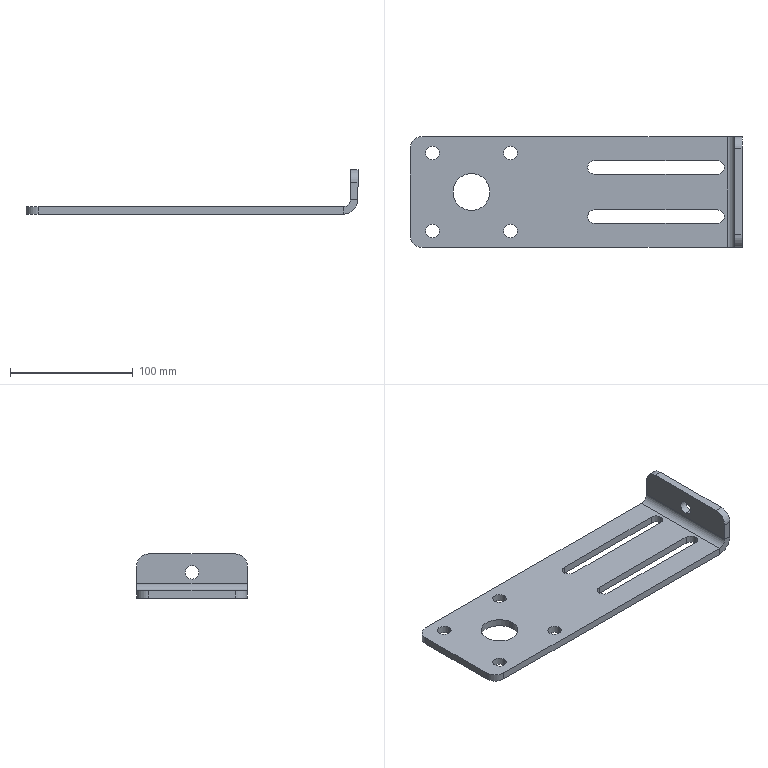Part | STEP file | Microwave Drying Flat Conveyor-CN2500x400-101-101 | 1 solid | 40 faces | box 270 x 90 x 36 mm | volume 137966 mm3 | cylinder 24 | plane 16 | commonest cylinder face diameters 11 x16 20 x4 30 x2 12 x1 24 x1
STEP:
#1=CARTESIAN_POINT('',(-99.75,26.75,-6.));
#2=VERTEX_POINT('',#1);
#3=CARTESIAN_POINT('',(-88.75,26.75,-6.));
#4=VERTEX_POINT('',#3);
#5=CARTESIAN_POINT('',(-94.25,26.75,-6.));
#6=DIRECTION('',(0.,0.,1.));
#7=DIRECTION('',(1.,0.,0.));
#8=AXIS2_PLACEMENT_3D('',#5,#6,#7);
#9=CIRCLE('',#8,5.5);
#10=EDGE_CURVE('',#2,#4,#9,.T.);
#11=ORIENTED_EDGE('',*,*,#10,.F.);
#12=CARTESIAN_POINT('',(-99.75,26.75,0.));
#13=VERTEX_POINT('',#12);
#14=CARTESIAN_POINT('',(-99.75,26.75,-10.));
#15=DIRECTION('',(0.,0.,1.));
#16=VECTOR('',#15,1000.);
#17=LINE('',#14,#16);
#18=EDGE_CURVE('',#2,#13,#17,.T.);
#19=ORIENTED_EDGE('',*,*,#18,.T.);
#20=CARTESIAN_POINT('',(-88.75,26.75,0.));
#21=VERTEX_POINT('',#20);
#22=CARTESIAN_POINT('',(-94.25,26.75,0.));
#23=DIRECTION('',(0.,0.,1.));
#24=DIRECTION('',(1.,0.,0.));
#25=AXIS2_PLACEMENT_3D('',#22,#23,#24);
#26=CIRCLE('',#25,5.5);
#27=EDGE_CURVE('',#13,#21,#26,.T.);
#28=ORIENTED_EDGE('',*,*,#27,.T.);
#29=CARTESIAN_POINT('',(-88.75,26.75,-10.));
#30=DIRECTION('',(0.,0.,1.));
#31=VECTOR('',#30,1000.);
#32=LINE('',#29,#31);
#33=EDGE_CURVE('',#4,#21,#32,.T.);
#34=ORIENTED_EDGE('',*,*,#33,.F.);
#35=EDGE_LOOP('',(#11,#19,#28,#34));
#36=FACE_OUTER_BOUND('',#35,.T.);
#37=CARTESIAN_POINT('',(-94.25,26.75,-10.));
#38=DIRECTION('',(0.,0.,1.));
#39=DIRECTION('',(1.,0.,0.));
#40=AXIS2_PLACEMENT_3D('',#37,#38,#39);
#41=CYLINDRICAL_SURFACE('',#40,5.5);
#42=ADVANCED_FACE('',(#36),#41,.F.);
#43=CARTESIAN_POINT('',(-36.25,26.75,-6.));
#44=VERTEX_POINT('',#43);
#45=CARTESIAN_POINT('',(-25.25,26.75,-6.));
#46=VERTEX_POINT('',#45);
#47=CARTESIAN_POINT('',(-30.75,26.75,-6.));
#48=DIRECTION('',(0.,0.,1.));
#49=DIRECTION('',(1.,0.,0.));
#50=AXIS2_PLACEMENT_3D('',#47,#48,#49);
#51=CIRCLE('',#50,5.5);
#52=EDGE_CURVE('',#44,#46,#51,.T.);
#53=ORIENTED_EDGE('',*,*,#52,.F.);
#54=CARTESIAN_POINT('',(-36.25,26.75,0.));
#55=VERTEX_POINT('',#54);
#56=CARTESIAN_POINT('',(-36.25,26.75,-10.));
#57=DIRECTION('',(0.,0.,1.));
#58=VECTOR('',#57,1000.);
#59=LINE('',#56,#58);
#60=EDGE_CURVE('',#44,#55,#59,.T.);
#61=ORIENTED_EDGE('',*,*,#60,.T.);
#62=CARTESIAN_POINT('',(-25.25,26.75,0.));
#63=VERTEX_POINT('',#62);
#64=CARTESIAN_POINT('',(-30.75,26.75,0.));
#65=DIRECTION('',(0.,0.,1.));
#66=DIRECTION('',(1.,0.,0.));
#67=AXIS2_PLACEMENT_3D('',#64,#65,#66);
#68=CIRCLE('',#67,5.5);
#69=EDGE_CURVE('',#55,#63,#68,.T.);
#70=ORIENTED_EDGE('',*,*,#69,.T.);
#71=CARTESIAN_POINT('',(-25.25,26.75,-10.));
#72=DIRECTION('',(0.,0.,1.));
#73=VECTOR('',#72,1000.);
#74=LINE('',#71,#73);
#75=EDGE_CURVE('',#46,#63,#74,.T.);
#76=ORIENTED_EDGE('',*,*,#75,.F.);
#77=EDGE_LOOP('',(#53,#61,#70,#76));
#78=FACE_OUTER_BOUND('',#77,.T.);
#79=CARTESIAN_POINT('',(-30.75,26.75,-10.));
#80=DIRECTION('',(0.,0.,1.));
#81=DIRECTION('',(1.,0.,0.));
#82=AXIS2_PLACEMENT_3D('',#79,#80,#81);
#83=CYLINDRICAL_SURFACE('',#82,5.5);
#84=ADVANCED_FACE('',(#78),#83,.F.);
#85=CARTESIAN_POINT('',(-36.25,-36.75,-6.));
#86=VERTEX_POINT('',#85);
#87=CARTESIAN_POINT('',(-25.25,-36.75,-6.));
#88=VERTEX_POINT('',#87);
#89=CARTESIAN_POINT('',(-30.75,-36.75,-6.));
#90=DIRECTION('',(0.,0.,1.));
#91=DIRECTION('',(1.,0.,0.));
#92=AXIS2_PLACEMENT_3D('',#89,#90,#91);
#93=CIRCLE('',#92,5.5);
#94=EDGE_CURVE('',#86,#88,#93,.T.);
#95=ORIENTED_EDGE('',*,*,#94,.F.);
#96=CARTESIAN_POINT('',(-36.25,-36.75,0.));
#97=VERTEX_POINT('',#96);
#98=CARTESIAN_POINT('',(-36.25,-36.75,-10.));
#99=DIRECTION('',(0.,0.,1.));
#100=VECTOR('',#99,1000.);
#101=LINE('',#98,#100);
#102=EDGE_CURVE('',#86,#97,#101,.T.);
#103=ORIENTED_EDGE('',*,*,#102,.T.);
#104=CARTESIAN_POINT('',(-25.25,-36.75,0.));
#105=VERTEX_POINT('',#104);
#106=CARTESIAN_POINT('',(-30.75,-36.75,0.));
#107=DIRECTION('',(0.,0.,1.));
#108=DIRECTION('',(1.,0.,0.));
#109=AXIS2_PLACEMENT_3D('',#106,#107,#108);
#110=CIRCLE('',#109,5.5);
#111=EDGE_CURVE('',#97,#105,#110,.T.);
#112=ORIENTED_EDGE('',*,*,#111,.T.);
#113=CARTESIAN_POINT('',(-25.25,-36.75,-10.));
#114=DIRECTION('',(0.,0.,1.));
#115=VECTOR('',#114,1000.);
#116=LINE('',#113,#115);
#117=EDGE_CURVE('',#88,#105,#116,.T.);
#118=ORIENTED_EDGE('',*,*,#117,.F.);
#119=EDGE_LOOP('',(#95,#103,#112,#118));
#120=FACE_OUTER_BOUND('',#119,.T.);
#121=CARTESIAN_POINT('',(-30.75,-36.75,-10.));
#122=DIRECTION('',(0.,0.,1.));
#123=DIRECTION('',(1.,0.,0.));
#124=AXIS2_PLACEMENT_3D('',#121,#122,#123);
#125=CYLINDRICAL_SURFACE('',#124,5.5);
#126=ADVANCED_FACE('',(#120),#125,.F.);
#127=CARTESIAN_POINT('',(-99.75,-36.75,-6.));
#128=VERTEX_POINT('',#127);
#129=CARTESIAN_POINT('',(-88.75,-36.75,-6.));
#130=VERTEX_POINT('',#129);
#131=CARTESIAN_POINT('',(-94.25,-36.75,-6.));
#132=DIRECTION('',(0.,0.,1.));
#133=DIRECTION('',(1.,0.,0.));
#134=AXIS2_PLACEMENT_3D('',#131,#132,#133);
#135=CIRCLE('',#134,5.5);
#136=EDGE_CURVE('',#128,#130,#135,.T.);
#137=ORIENTED_EDGE('',*,*,#136,.F.);
#138=CARTESIAN_POINT('',(-99.75,-36.75,0.));
#139=VERTEX_POINT('',#138);
#140=CARTESIAN_POINT('',(-99.75,-36.75,-10.));
#141=DIRECTION('',(0.,0.,1.));
#142=VECTOR('',#141,1000.);
#143=LINE('',#140,#142);
#144=EDGE_CURVE('',#128,#139,#143,.T.);
#145=ORIENTED_EDGE('',*,*,#144,.T.);
#146=CARTESIAN_POINT('',(-88.75,-36.75,0.));
#147=VERTEX_POINT('',#146);
#148=CARTESIAN_POINT('',(-94.25,-36.75,0.));
#149=DIRECTION('',(0.,0.,1.));
#150=DIRECTION('',(1.,0.,0.));
#151=AXIS2_PLACEMENT_3D('',#148,#149,#150);
#152=CIRCLE('',#151,5.5);
#153=EDGE_CURVE('',#139,#147,#152,.T.);
#154=ORIENTED_EDGE('',*,*,#153,.T.);
#155=CARTESIAN_POINT('',(-88.75,-36.75,-10.));
#156=DIRECTION('',(0.,0.,1.));
#157=VECTOR('',#156,1000.);
#158=LINE('',#155,#157);
#159=EDGE_CURVE('',#130,#147,#158,.T.);
#160=ORIENTED_EDGE('',*,*,#159,.F.);
#161=EDGE_LOOP('',(#137,#145,#154,#160));
#162=FACE_OUTER_BOUND('',#161,.T.);
#163=CARTESIAN_POINT('',(-94.25,-36.75,-10.));
#164=DIRECTION('',(0.,0.,1.));
#165=DIRECTION('',(1.,0.,0.));
#166=AXIS2_PLACEMENT_3D('',#163,#164,#165);
#167=CYLINDRICAL_SURFACE('',#166,5.5);
#168=ADVANCED_FACE('',(#162),#167,.F.);
#169=CARTESIAN_POINT('',(-77.5,-5.,-6.));
#170=VERTEX_POINT('',#169);
#171=CARTESIAN_POINT('',(-47.5,-5.,-6.));
#172=VERTEX_POINT('',#171);
#173=CARTESIAN_POINT('',(-62.5,-5.,-6.));
#174=DIRECTION('',(0.,0.,1.));
#175=DIRECTION('',(1.,0.,0.));
#176=AXIS2_PLACEMENT_3D('',#173,#174,#175);
#177=CIRCLE('',#176,15.);
#178=EDGE_CURVE('',#170,#172,#177,.T.);
#179=ORIENTED_EDGE('',*,*,#178,.F.);
#180=CARTESIAN_POINT('',(-77.5,-5.,0.));
#181=VERTEX_POINT('',#180);
#182=CARTESIAN_POINT('',(-77.5,-5.,-10.));
#183=DIRECTION('',(0.,0.,1.));
#184=VECTOR('',#183,1000.);
#185=LINE('',#182,#184);
#186=EDGE_CURVE('',#170,#181,#185,.T.);
#187=ORIENTED_EDGE('',*,*,#186,.T.);
#188=CARTESIAN_POINT('',(-47.5,-5.,0.));
#189=VERTEX_POINT('',#188);
#190=CARTESIAN_POINT('',(-62.5,-5.,0.));
#191=DIRECTION('',(0.,0.,1.));
#192=DIRECTION('',(1.,0.,0.));
#193=AXIS2_PLACEMENT_3D('',#190,#191,#192);
#194=CIRCLE('',#193,15.);
#195=EDGE_CURVE('',#181,#189,#194,.T.);
#196=ORIENTED_EDGE('',*,*,#195,.T.);
#197=CARTESIAN_POINT('',(-47.5,-5.,-10.));
#198=DIRECTION('',(0.,0.,1.));
#199=VECTOR('',#198,1000.);
#200=LINE('',#197,#199);
#201=EDGE_CURVE('',#172,#189,#200,.T.);
#202=ORIENTED_EDGE('',*,*,#201,.F.);
#203=EDGE_LOOP('',(#179,#187,#196,#202));
#204=FACE_OUTER_BOUND('',#203,.T.);
#205=CARTESIAN_POINT('',(-62.5,-5.,-10.));
#206=DIRECTION('',(0.,0.,1.));
#207=DIRECTION('',(1.,0.,0.));
#208=AXIS2_PLACEMENT_3D('',#205,#206,#207);
#209=CYLINDRICAL_SURFACE('',#208,15.);
#210=ADVANCED_FACE('',(#204),#209,.F.);
#211=CARTESIAN_POINT('',(151.5,-5.,9.5));
#212=VERTEX_POINT('',#211);
#213=CARTESIAN_POINT('',(151.5,-5.,20.5));
#214=VERTEX_POINT('',#213);
#215=CARTESIAN_POINT('',(151.5,-5.,15.));
#216=DIRECTION('',(-1.,0.,0.));
#217=DIRECTION('',(0.,0.,1.));
#218=AXIS2_PLACEMENT_3D('',#215,#216,#217);
#219=CIRCLE('',#218,5.5);
#220=EDGE_CURVE('',#212,#214,#219,.T.);
#221=ORIENTED_EDGE('',*,*,#220,.T.);
#222=CARTESIAN_POINT('',(157.5,-5.,20.5));
#223=VERTEX_POINT('',#222);
#224=CARTESIAN_POINT('',(147.5,-5.,20.5));
#225=DIRECTION('',(1.,0.,0.));
#226=VECTOR('',#225,1000.);
#227=LINE('',#224,#226);
#228=EDGE_CURVE('',#214,#223,#227,.T.);
#229=ORIENTED_EDGE('',*,*,#228,.T.);
#230=CARTESIAN_POINT('',(157.5,-5.,9.5));
#231=VERTEX_POINT('',#230);
#232=CARTESIAN_POINT('',(157.5,-5.,15.));
#233=DIRECTION('',(1.,0.,0.));
#234=DIRECTION('',(0.,0.,-1.));
#235=AXIS2_PLACEMENT_3D('',#232,#233,#234);
#236=CIRCLE('',#235,5.5);
#237=EDGE_CURVE('',#223,#231,#236,.T.);
#238=ORIENTED_EDGE('',*,*,#237,.T.);
#239=CARTESIAN_POINT('',(147.5,-5.,9.5));
#240=DIRECTION('',(1.,0.,0.));
#241=VECTOR('',#240,1000.);
#242=LINE('',#239,#241);
#243=EDGE_CURVE('',#212,#231,#242,.T.);
#244=ORIENTED_EDGE('',*,*,#243,.F.);
#245=EDGE_LOOP('',(#221,#229,#238,#244));
#246=FACE_OUTER_BOUND('',#245,.T.);
#247=CARTESIAN_POINT('',(147.5,-5.,15.));
#248=DIRECTION('',(1.,0.,0.));
#249=DIRECTION('',(0.,0.,-1.));
#250=AXIS2_PLACEMENT_3D('',#247,#248,#249);
#251=CYLINDRICAL_SURFACE('',#250,5.5);
#252=ADVANCED_FACE('',(#246),#251,.F.);
#253=CARTESIAN_POINT('',(143.,15.,-6.));
#254=VERTEX_POINT('',#253);
#255=CARTESIAN_POINT('',(137.5,20.5,-6.));
#256=VERTEX_POINT('',#255);
#257=CARTESIAN_POINT('',(137.5,15.,-6.));
#258=DIRECTION('',(0.,0.,1.));
#259=DIRECTION('',(1.,0.,0.));
#260=AXIS2_PLACEMENT_3D('',#257,#258,#259);
#261=CIRCLE('',#260,5.5);
#262=EDGE_CURVE('',#254,#256,#261,.T.);
#263=ORIENTED_EDGE('',*,*,#262,.F.);
#264=CARTESIAN_POINT('',(143.,15.,0.));
#265=VERTEX_POINT('',#264);
#266=CARTESIAN_POINT('',(143.,15.,-10.));
#267=DIRECTION('',(0.,0.,1.));
#268=VECTOR('',#267,1000.);
#269=LINE('',#266,#268);
#270=EDGE_CURVE('',#254,#265,#269,.T.);
#271=ORIENTED_EDGE('',*,*,#270,.T.);
#272=CARTESIAN_POINT('',(137.5,20.5,0.));
#273=VERTEX_POINT('',#272);
#274=CARTESIAN_POINT('',(137.5,15.,0.));
#275=DIRECTION('',(0.,0.,1.));
#276=DIRECTION('',(1.,0.,0.));
#277=AXIS2_PLACEMENT_3D('',#274,#275,#276);
#278=CIRCLE('',#277,5.5);
#279=EDGE_CURVE('',#265,#273,#278,.T.);
#280=ORIENTED_EDGE('',*,*,#279,.T.);
#281=CARTESIAN_POINT('',(137.5,20.5,-10.));
#282=DIRECTION('',(0.,0.,1.));
#283=VECTOR('',#282,1000.);
#284=LINE('',#281,#283);
#285=EDGE_CURVE('',#256,#273,#284,.T.);
#286=ORIENTED_EDGE('',*,*,#285,.F.);
#287=EDGE_LOOP('',(#263,#271,#280,#286));
#288=FACE_OUTER_BOUND('',#287,.T.);
#289=CARTESIAN_POINT('',(137.5,15.,-10.));
#290=DIRECTION('',(0.,0.,1.));
#291=DIRECTION('',(1.,0.,0.));
#292=AXIS2_PLACEMENT_3D('',#289,#290,#291);
#293=CYLINDRICAL_SURFACE('',#292,5.5);
#294=ADVANCED_FACE('',(#288),#293,.F.);
#295=CARTESIAN_POINT('',(143.,-25.,-6.));
#296=VERTEX_POINT('',#295);
#297=CARTESIAN_POINT('',(137.5,-19.5,-6.));
#298=VERTEX_POINT('',#297);
#299=CARTESIAN_POINT('',(137.5,-25.,-6.));
#300=DIRECTION('',(0.,0.,1.));
#301=DIRECTION('',(1.,0.,0.));
#302=AXIS2_PLACEMENT_3D('',#299,#300,#301);
#303=CIRCLE('',#302,5.5);
#304=EDGE_CURVE('',#296,#298,#303,.T.);
#305=ORIENTED_EDGE('',*,*,#304,.F.);
#306=CARTESIAN_POINT('',(143.,-25.,0.));
#307=VERTEX_POINT('',#306);
#308=CARTESIAN_POINT('',(143.,-25.,-10.));
#309=DIRECTION('',(0.,0.,1.));
#310=VECTOR('',#309,1000.);
#311=LINE('',#308,#310);
#312=EDGE_CURVE('',#296,#307,#311,.T.);
#313=ORIENTED_EDGE('',*,*,#312,.T.);
#314=CARTESIAN_POINT('',(137.5,-19.5,0.));
#315=VERTEX_POINT('',#314);
#316=CARTESIAN_POINT('',(137.5,-25.,0.));
#317=DIRECTION('',(0.,0.,1.));
#318=DIRECTION('',(1.,0.,0.));
#319=AXIS2_PLACEMENT_3D('',#316,#317,#318);
#320=CIRCLE('',#319,5.5);
#321=EDGE_CURVE('',#307,#315,#320,.T.);
#322=ORIENTED_EDGE('',*,*,#321,.T.);
#323=CARTESIAN_POINT('',(137.5,-19.5,-10.));
#324=DIRECTION('',(0.,0.,1.));
#325=VECTOR('',#324,1000.);
#326=LINE('',#323,#325);
#327=EDGE_CURVE('',#298,#315,#326,.T.);
#328=ORIENTED_EDGE('',*,*,#327,.F.);
#329=EDGE_LOOP('',(#305,#313,#322,#328));
#330=FACE_OUTER_BOUND('',#329,.T.);
#331=CARTESIAN_POINT('',(137.5,-25.,-10.));
#332=DIRECTION('',(0.,0.,1.));
#333=DIRECTION('',(1.,0.,0.));
#334=AXIS2_PLACEMENT_3D('',#331,#332,#333);
#335=CYLINDRICAL_SURFACE('',#334,5.5);
#336=ADVANCED_FACE('',(#330),#335,.F.);
#337=CARTESIAN_POINT('',(145.5,40.,0.));
#338=VERTEX_POINT('',#337);
#339=CARTESIAN_POINT('',(-102.5,40.,0.));
#340=VERTEX_POINT('',#339);
#341=CARTESIAN_POINT('',(-102.5,40.,0.));
#342=DIRECTION('',(-1.,0.,0.));
#343=VECTOR('',#342,1000.);
#344=LINE('',#341,#343);
#345=EDGE_CURVE('',#338,#340,#344,.T.);
#346=ORIENTED_EDGE('',*,*,#345,.F.);
#347=CARTESIAN_POINT('',(145.5,40.,-6.));
#348=VERTEX_POINT('',#347);
#349=CARTESIAN_POINT('',(145.5,40.,0.));
#350=DIRECTION('',(0.,0.,-1.));
#351=VECTOR('',#350,1000.);
#352=LINE('',#349,#351);
#353=EDGE_CURVE('',#338,#348,#352,.T.);
#354=ORIENTED_EDGE('',*,*,#353,.T.);
#355=CARTESIAN_POINT('',(-102.5,40.,-6.));
#356=VERTEX_POINT('',#355);
#357=CARTESIAN_POINT('',(-102.5,40.,-6.));
#358=DIRECTION('',(-1.,0.,0.));
#359=VECTOR('',#358,1000.);
#360=LINE('',#357,#359);
#361=EDGE_CURVE('',#348,#356,#360,.T.);
#362=ORIENTED_EDGE('',*,*,#361,.T.);
#363=CARTESIAN_POINT('',(-102.5,40.,-6.));
#364=DIRECTION('',(0.,0.,1.));
#365=VECTOR('',#364,1000.);
#366=LINE('',#363,#365);
#367=EDGE_CURVE('',#356,#340,#366,.T.);
#368=ORIENTED_EDGE('',*,*,#367,.T.);
#369=EDGE_LOOP('',(#346,#354,#362,#368));
#370=FACE_OUTER_BOUND('',#369,.T.);
#371=CARTESIAN_POINT('',(-102.5,40.,-6.));
#372=DIRECTION('',(0.,1.,0.));
#373=DIRECTION('',(0.,0.,1.));
#374=AXIS2_PLACEMENT_3D('',#371,#372,#373);
#375=PLANE('',#374);
#376=ADVANCED_FACE('',(#370),#375,.T.);
#377=CARTESIAN_POINT('',(-94.25,26.75,-6.));
#378=DIRECTION('',(0.,0.,1.));
#379=DIRECTION('',(1.,0.,0.));
#380=AXIS2_PLACEMENT_3D('',#377,#378,#379);
#381=CIRCLE('',#380,5.5);
#382=EDGE_CURVE('',#4,#2,#381,.T.);
#383=ORIENTED_EDGE('',*,*,#382,.T.);
#384=ORIENTED_EDGE('',*,*,#10,.T.);
#385=EDGE_LOOP('',(#383,#384));
#386=FACE_BOUND('',#385,.T.);
#387=CARTESIAN_POINT('',(-30.75,26.75,-6.));
#388=DIRECTION('',(0.,0.,1.));
#389=DIRECTION('',(1.,0.,0.));
#390=AXIS2_PLACEMENT_3D('',#387,#388,#389);
#391=CIRCLE('',#390,5.5);
#392=EDGE_CURVE('',#46,#44,#391,.T.);
#393=ORIENTED_EDGE('',*,*,#392,.T.);
#394=ORIENTED_EDGE('',*,*,#52,.T.);
#395=EDGE_LOOP('',(#393,#394));
#396=FACE_BOUND('',#395,.T.);
#397=CARTESIAN_POINT('',(-30.75,-36.75,-6.));
#398=DIRECTION('',(0.,0.,1.));
#399=DIRECTION('',(1.,0.,0.));
#400=AXIS2_PLACEMENT_3D('',#397,#398,#399);
#401=CIRCLE('',#400,5.5);
#402=EDGE_CURVE('',#88,#86,#401,.T.);
#403=ORIENTED_EDGE('',*,*,#402,.T.);
#404=ORIENTED_EDGE('',*,*,#94,.T.);
#405=EDGE_LOOP('',(#403,#404));
#406=FACE_BOUND('',#405,.T.);
#407=CARTESIAN_POINT('',(-94.25,-36.75,-6.));
#408=DIRECTION('',(0.,0.,1.));
#409=DIRECTION('',(1.,0.,0.));
#410=AXIS2_PLACEMENT_3D('',#407,#408,#409);
#411=CIRCLE('',#410,5.5);
#412=EDGE_CURVE('',#130,#128,#411,.T.);
#413=ORIENTED_EDGE('',*,*,#412,.T.);
#414=ORIENTED_EDGE('',*,*,#136,.T.);
#415=EDGE_LOOP('',(#413,#414));
#416=FACE_BOUND('',#415,.T.);
#417=CARTESIAN_POINT('',(-62.5,-5.,-6.));
#418=DIRECTION('',(0.,0.,1.));
#419=DIRECTION('',(1.,0.,0.));
#420=AXIS2_PLACEMENT_3D('',#417,#418,#419);
#421=CIRCLE('',#420,15.);
#422=EDGE_CURVE('',#172,#170,#421,.T.);
#423=ORIENTED_EDGE('',*,*,#422,.T.);
#424=ORIENTED_EDGE('',*,*,#178,.T.);
#425=EDGE_LOOP('',(#423,#424));
#426=FACE_BOUND('',#425,.T.);
#427=CARTESIAN_POINT('',(37.5,20.5,-6.));
#428=VERTEX_POINT('',#427);
#429=CARTESIAN_POINT('',(-102.5,20.5,-6.));
#430=DIRECTION('',(-1.,0.,0.));
#431=VECTOR('',#430,1000.);
#432=LINE('',#429,#431);
#433=EDGE_CURVE('',#256,#428,#432,.T.);
#434=ORIENTED_EDGE('',*,*,#433,.T.);
#435=CARTESIAN_POINT('',(37.5,9.5,-6.));
#436=VERTEX_POINT('',#435);
#437=CARTESIAN_POINT('',(37.5,15.,-6.));
#438=DIRECTION('',(0.,0.,1.));
#439=DIRECTION('',(1.,0.,0.));
#440=AXIS2_PLACEMENT_3D('',#437,#438,#439);
#441=CIRCLE('',#440,5.5);
#442=EDGE_CURVE('',#428,#436,#441,.T.);
#443=ORIENTED_EDGE('',*,*,#442,.T.);
#444=CARTESIAN_POINT('',(137.5,9.5,-6.));
#445=VERTEX_POINT('',#444);
#446=CARTESIAN_POINT('',(-102.5,9.5,-6.));
#447=DIRECTION('',(1.,0.,0.));
#448=VECTOR('',#447,1000.);
#449=LINE('',#446,#448);
#450=EDGE_CURVE('',#436,#445,#449,.T.);
#451=ORIENTED_EDGE('',*,*,#450,.T.);
#452=CARTESIAN_POINT('',(137.5,15.,-6.));
#453=DIRECTION('',(0.,0.,1.));
#454=DIRECTION('',(1.,0.,0.));
#455=AXIS2_PLACEMENT_3D('',#452,#453,#454);
#456=CIRCLE('',#455,5.5);
#457=EDGE_CURVE('',#445,#254,#456,.T.);
#458=ORIENTED_EDGE('',*,*,#457,.T.);
#459=ORIENTED_EDGE('',*,*,#262,.T.);
#460=EDGE_LOOP('',(#434,#443,#451,#458,#459));
#461=FACE_BOUND('',#460,.T.);
#462=CARTESIAN_POINT('',(37.5,-19.5,-6.));
#463=VERTEX_POINT('',#462);
#464=CARTESIAN_POINT('',(-102.5,-19.5,-6.));
#465=DIRECTION('',(-1.,0.,0.));
#466=VECTOR('',#465,1000.);
#467=LINE('',#464,#466);
#468=EDGE_CURVE('',#298,#463,#467,.T.);
#469=ORIENTED_EDGE('',*,*,#468,.T.);
#470=CARTESIAN_POINT('',(37.5,-30.5,-6.));
#471=VERTEX_POINT('',#470);
#472=CARTESIAN_POINT('',(37.5,-25.,-6.));
#473=DIRECTION('',(0.,0.,1.));
#474=DIRECTION('',(1.,0.,0.));
#475=AXIS2_PLACEMENT_3D('',#472,#473,#474);
#476=CIRCLE('',#475,5.5);
#477=EDGE_CURVE('',#463,#471,#476,.T.);
#478=ORIENTED_EDGE('',*,*,#477,.T.);
#479=CARTESIAN_POINT('',(137.5,-30.5,-6.));
#480=VERTEX_POINT('',#479);
#481=CARTESIAN_POINT('',(-102.5,-30.5,-6.));
#482=DIRECTION('',(1.,0.,0.));
#483=VECTOR('',#482,1000.);
#484=LINE('',#481,#483);
#485=EDGE_CURVE('',#471,#480,#484,.T.);
#486=ORIENTED_EDGE('',*,*,#485,.T.);
#487=CARTESIAN_POINT('',(137.5,-25.,-6.));
#488=DIRECTION('',(0.,0.,1.));
#489=DIRECTION('',(1.,0.,0.));
#490=AXIS2_PLACEMENT_3D('',#487,#488,#489);
#491=CIRCLE('',#490,5.5);
#492=EDGE_CURVE('',#480,#296,#491,.T.);
#493=ORIENTED_EDGE('',*,*,#492,.T.);
#494=ORIENTED_EDGE('',*,*,#304,.T.);
#495=EDGE_LOOP('',(#469,#478,#486,#493,#494));
#496=FACE_BOUND('',#495,.T.);
#497=CARTESIAN_POINT('',(145.5,-50.,-6.));
#498=VERTEX_POINT('',#497);
#499=CARTESIAN_POINT('',(145.5,40.,-6.));
#500=DIRECTION('',(0.,-1.,0.));
#501=VECTOR('',#500,1000.);
#502=LINE('',#499,#501);
#503=EDGE_CURVE('',#348,#498,#502,.T.);
#504=ORIENTED_EDGE('',*,*,#503,.T.);
#505=CARTESIAN_POINT('',(-102.5,-50.,-6.));
#506=VERTEX_POINT('',#505);
#507=CARTESIAN_POINT('',(-102.5,-50.,-6.));
#508=DIRECTION('',(1.,0.,0.));
#509=VECTOR('',#508,1000.);
#510=LINE('',#507,#509);
#511=EDGE_CURVE('',#506,#498,#510,.T.);
#512=ORIENTED_EDGE('',*,*,#511,.F.);
#513=CARTESIAN_POINT('',(-112.5,-40.,-6.));
#514=VERTEX_POINT('',#513);
#515=CARTESIAN_POINT('',(-102.5,-40.,-6.));
#516=DIRECTION('',(0.,0.,1.));
#517=DIRECTION('',(1.,0.,0.));
#518=AXIS2_PLACEMENT_3D('',#515,#516,#517);
#519=CIRCLE('',#518,10.);
#520=EDGE_CURVE('',#514,#506,#519,.T.);
#521=ORIENTED_EDGE('',*,*,#520,.F.);
#522=CARTESIAN_POINT('',(-112.5,30.,-6.));
#523=VERTEX_POINT('',#522);
#524=CARTESIAN_POINT('',(-112.5,30.,-6.));
#525=DIRECTION('',(0.,-1.,0.));
#526=VECTOR('',#525,1000.);
#527=LINE('',#524,#526);
#528=EDGE_CURVE('',#523,#514,#527,.T.);
#529=ORIENTED_EDGE('',*,*,#528,.F.);
#530=CARTESIAN_POINT('',(-102.5,30.,-6.));
#531=DIRECTION('',(0.,0.,1.));
#532=DIRECTION('',(1.,0.,0.));
#533=AXIS2_PLACEMENT_3D('',#530,#531,#532);
#534=CIRCLE('',#533,10.);
#535=EDGE_CURVE('',#356,#523,#534,.T.);
#536=ORIENTED_EDGE('',*,*,#535,.F.);
#537=ORIENTED_EDGE('',*,*,#361,.F.);
#538=EDGE_LOOP('',(#504,#512,#521,#529,#536,#537));
#539=FACE_OUTER_BOUND('',#538,.T.);
#540=CARTESIAN_POINT('',(-102.5,-40.,-6.));
#541=DIRECTION('',(0.,0.,1.));
#542=DIRECTION('',(1.,0.,0.));
#543=AXIS2_PLACEMENT_3D('',#540,#541,#542);
#544=PLANE('',#543);
#545=ADVANCED_FACE('',(#386,#396,#406,#416,#426,#461,#496,#539),#544,.F.);
#546=CARTESIAN_POINT('',(-94.25,26.75,0.));
#547=DIRECTION('',(0.,0.,1.));
#548=DIRECTION('',(1.,0.,0.));
#549=AXIS2_PLACEMENT_3D('',#546,#547,#548);
#550=CIRCLE('',#549,5.5);
#551=EDGE_CURVE('',#21,#13,#550,.T.);
#552=ORIENTED_EDGE('',*,*,#551,.F.);
#553=ORIENTED_EDGE('',*,*,#27,.F.);
#554=EDGE_LOOP('',(#552,#553));
#555=FACE_BOUND('',#554,.T.);
#556=CARTESIAN_POINT('',(-30.75,26.75,0.));
#557=DIRECTION('',(0.,0.,1.));
#558=DIRECTION('',(1.,0.,0.));
#559=AXIS2_PLACEMENT_3D('',#556,#557,#558);
#560=CIRCLE('',#559,5.5);
#561=EDGE_CURVE('',#63,#55,#560,.T.);
#562=ORIENTED_EDGE('',*,*,#561,.F.);
#563=ORIENTED_EDGE('',*,*,#69,.F.);
#564=EDGE_LOOP('',(#562,#563));
#565=FACE_BOUND('',#564,.T.);
#566=CARTESIAN_POINT('',(-30.75,-36.75,0.));
#567=DIRECTION('',(0.,0.,1.));
#568=DIRECTION('',(1.,0.,0.));
#569=AXIS2_PLACEMENT_3D('',#566,#567,#568);
#570=CIRCLE('',#569,5.5);
#571=EDGE_CURVE('',#105,#97,#570,.T.);
#572=ORIENTED_EDGE('',*,*,#571,.F.);
#573=ORIENTED_EDGE('',*,*,#111,.F.);
#574=EDGE_LOOP('',(#572,#573));
#575=FACE_BOUND('',#574,.T.);
#576=CARTESIAN_POINT('',(-94.25,-36.75,0.));
#577=DIRECTION('',(0.,0.,1.));
#578=DIRECTION('',(1.,0.,0.));
#579=AXIS2_PLACEMENT_3D('',#576,#577,#578);
#580=CIRCLE('',#579,5.5);
#581=EDGE_CURVE('',#147,#139,#580,.T.);
#582=ORIENTED_EDGE('',*,*,#581,.F.);
#583=ORIENTED_EDGE('',*,*,#153,.F.);
#584=EDGE_LOOP('',(#582,#583));
#585=FACE_BOUND('',#584,.T.);
#586=CARTESIAN_POINT('',(-62.5,-5.,0.));
#587=DIRECTION('',(0.,0.,1.));
#588=DIRECTION('',(1.,0.,0.));
#589=AXIS2_PLACEMENT_3D('',#586,#587,#588);
#590=CIRCLE('',#589,15.);
#591=EDGE_CURVE('',#189,#181,#590,.T.);
#592=ORIENTED_EDGE('',*,*,#591,.F.);
#593=ORIENTED_EDGE('',*,*,#195,.F.);
#594=EDGE_LOOP('',(#592,#593));
#595=FACE_BOUND('',#594,.T.);
#596=CARTESIAN_POINT('',(37.5,20.5,0.));
#597=VERTEX_POINT('',#596);
#598=CARTESIAN_POINT('',(37.5,9.5,0.));
#599=VERTEX_POINT('',#598);
#600=CARTESIAN_POINT('',(37.5,15.,0.));
#601=DIRECTION('',(0.,0.,1.));
#602=DIRECTION('',(1.,0.,0.));
#603=AXIS2_PLACEMENT_3D('',#600,#601,#602);
#604=CIRCLE('',#603,5.5);
#605=EDGE_CURVE('',#597,#599,#604,.T.);
#606=ORIENTED_EDGE('',*,*,#605,.F.);
#607=CARTESIAN_POINT('',(37.5,20.5,0.));
#608=DIRECTION('',(-1.,0.,0.));
#609=VECTOR('',#608,1000.);
#610=LINE('',#607,#609);
#611=EDGE_CURVE('',#273,#597,#610,.T.);
#612=ORIENTED_EDGE('',*,*,#611,.F.);
#613=ORIENTED_EDGE('',*,*,#279,.F.);
#614=CARTESIAN_POINT('',(137.5,9.5,0.));
#615=VERTEX_POINT('',#614);
#616=CARTESIAN_POINT('',(137.5,15.,0.));
#617=DIRECTION('',(0.,0.,1.));
#618=DIRECTION('',(1.,0.,0.));
#619=AXIS2_PLACEMENT_3D('',#616,#617,#618);
#620=CIRCLE('',#619,5.5);
#621=EDGE_CURVE('',#615,#265,#620,.T.);
#622=ORIENTED_EDGE('',*,*,#621,.F.);
#623=CARTESIAN_POINT('',(37.5,9.5,0.));
#624=DIRECTION('',(1.,0.,0.));
#625=VECTOR('',#624,1000.);
#626=LINE('',#623,#625);
#627=EDGE_CURVE('',#599,#615,#626,.T.);
#628=ORIENTED_EDGE('',*,*,#627,.F.);
#629=EDGE_LOOP('',(#606,#612,#613,#622,#628));
#630=FACE_BOUND('',#629,.T.);
#631=CARTESIAN_POINT('',(37.5,-19.5,0.));
#632=VERTEX_POINT('',#631);
#633=CARTESIAN_POINT('',(37.5,-30.5,0.));
#634=VERTEX_POINT('',#633);
#635=CARTESIAN_POINT('',(37.5,-25.,0.));
#636=DIRECTION('',(0.,0.,1.));
#637=DIRECTION('',(1.,0.,0.));
#638=AXIS2_PLACEMENT_3D('',#635,#636,#637);
#639=CIRCLE('',#638,5.5);
#640=EDGE_CURVE('',#632,#634,#639,.T.);
#641=ORIENTED_EDGE('',*,*,#640,.F.);
#642=CARTESIAN_POINT('',(37.5,-19.5,0.));
#643=DIRECTION('',(-1.,0.,0.));
#644=VECTOR('',#643,1000.);
#645=LINE('',#642,#644);
#646=EDGE_CURVE('',#315,#632,#645,.T.);
#647=ORIENTED_EDGE('',*,*,#646,.F.);
#648=ORIENTED_EDGE('',*,*,#321,.F.);
#649=CARTESIAN_POINT('',(137.5,-30.5,0.));
#650=VERTEX_POINT('',#649);
#651=CARTESIAN_POINT('',(137.5,-25.,0.));
#652=DIRECTION('',(0.,0.,1.));
#653=DIRECTION('',(1.,0.,0.));
#654=AXIS2_PLACEMENT_3D('',#651,#652,#653);
#655=CIRCLE('',#654,5.5);
#656=EDGE_CURVE('',#650,#307,#655,.T.);
#657=ORIENTED_EDGE('',*,*,#656,.F.);
#658=CARTESIAN_POINT('',(37.5,-30.5,0.));
#659=DIRECTION('',(1.,0.,0.));
#660=VECTOR('',#659,1000.);
#661=LINE('',#658,#660);
#662=EDGE_CURVE('',#634,#650,#661,.T.);
#663=ORIENTED_EDGE('',*,*,#662,.F.);
#664=EDGE_LOOP('',(#641,#647,#648,#657,#663));
#665=FACE_BOUND('',#664,.T.);
#666=CARTESIAN_POINT('',(-102.5,-50.,0.));
#667=VERTEX_POINT('',#666);
#668=CARTESIAN_POINT('',(145.5,-50.,0.));
#669=VERTEX_POINT('',#668);
#670=CARTESIAN_POINT('',(-102.5,-50.,0.));
#671=DIRECTION('',(1.,0.,0.));
#672=VECTOR('',#671,1000.);
#673=LINE('',#670,#672);
#674=EDGE_CURVE('',#667,#669,#673,.T.);
#675=ORIENTED_EDGE('',*,*,#674,.T.);
#676=CARTESIAN_POINT('',(145.5,40.,0.));
#677=DIRECTION('',(0.,-1.,0.));
#678=VECTOR('',#677,1000.);
#679=LINE('',#676,#678);
#680=EDGE_CURVE('',#338,#669,#679,.T.);
#681=ORIENTED_EDGE('',*,*,#680,.F.);
#682=ORIENTED_EDGE('',*,*,#345,.T.);
#683=CARTESIAN_POINT('',(-112.5,30.,0.));
#684=VERTEX_POINT('',#683);
#685=CARTESIAN_POINT('',(-102.5,30.,0.));
#686=DIRECTION('',(0.,0.,1.));
#687=DIRECTION('',(1.,0.,0.));
#688=AXIS2_PLACEMENT_3D('',#685,#686,#687);
#689=CIRCLE('',#688,10.);
#690=EDGE_CURVE('',#340,#684,#689,.T.);
#691=ORIENTED_EDGE('',*,*,#690,.T.);
#692=CARTESIAN_POINT('',(-112.5,-40.,0.));
#693=VERTEX_POINT('',#692);
#694=CARTESIAN_POINT('',(-112.5,30.,0.));
#695=DIRECTION('',(0.,-1.,0.));
#696=VECTOR('',#695,1000.);
#697=LINE('',#694,#696);
#698=EDGE_CURVE('',#684,#693,#697,.T.);
#699=ORIENTED_EDGE('',*,*,#698,.T.);
#700=CARTESIAN_POINT('',(-102.5,-40.,0.));
#701=DIRECTION('',(0.,0.,1.));
#702=DIRECTION('',(1.,0.,0.));
#703=AXIS2_PLACEMENT_3D('',#700,#701,#702);
#704=CIRCLE('',#703,10.);
#705=EDGE_CURVE('',#693,#667,#704,.T.);
#706=ORIENTED_EDGE('',*,*,#705,.T.);
#707=EDGE_LOOP('',(#675,#681,#682,#691,#699,#706));
#708=FACE_OUTER_BOUND('',#707,.T.);
#709=CARTESIAN_POINT('',(-102.5,-40.,0.));
#710=DIRECTION('',(0.,0.,1.));
#711=DIRECTION('',(1.,0.,0.));
#712=AXIS2_PLACEMENT_3D('',#709,#710,#711);
#713=PLANE('',#712);
#714=ADVANCED_FACE('',(#555,#565,#575,#585,#595,#630,#665,#708),#713,.T.);
#715=CARTESIAN_POINT('',(145.5,-50.,0.));
#716=DIRECTION('',(0.,0.,-1.));
#717=VECTOR('',#716,1000.);
#718=LINE('',#715,#717);
#719=EDGE_CURVE('',#669,#498,#718,.T.);
#720=ORIENTED_EDGE('',*,*,#719,.F.);
#721=ORIENTED_EDGE('',*,*,#674,.F.);
#722=CARTESIAN_POINT('',(-102.5,-50.,-6.));
#723=DIRECTION('',(0.,0.,1.));
#724=VECTOR('',#723,1000.);
#725=LINE('',#722,#724);
#726=EDGE_CURVE('',#506,#667,#725,.T.);
#727=ORIENTED_EDGE('',*,*,#726,.F.);
#728=ORIENTED_EDGE('',*,*,#511,.T.);
#729=EDGE_LOOP('',(#720,#721,#727,#728));
#730=FACE_OUTER_BOUND('',#729,.T.);
#731=CARTESIAN_POINT('',(-102.5,-50.,-6.));
#732=DIRECTION('',(0.,-1.,0.));
#733=DIRECTION('',(1.,0.,0.));
#734=AXIS2_PLACEMENT_3D('',#731,#732,#733);
#735=PLANE('',#734);
#736=ADVANCED_FACE('',(#730),#735,.T.);
#737=ORIENTED_EDGE('',*,*,#705,.F.);
#738=CARTESIAN_POINT('',(-112.5,-40.,-6.));
#739=DIRECTION('',(0.,0.,1.));
#740=VECTOR('',#739,1000.);
#741=LINE('',#738,#740);
#742=EDGE_CURVE('',#514,#693,#741,.T.);
#743=ORIENTED_EDGE('',*,*,#742,.F.);
#744=ORIENTED_EDGE('',*,*,#520,.T.);
#745=ORIENTED_EDGE('',*,*,#726,.T.);
#746=EDGE_LOOP('',(#737,#743,#744,#745));
#747=FACE_OUTER_BOUND('',#746,.T.);
#748=CARTESIAN_POINT('',(-102.5,-40.,-6.));
#749=DIRECTION('',(0.,0.,1.));
#750=DIRECTION('',(1.,0.,0.));
#751=AXIS2_PLACEMENT_3D('',#748,#749,#750);
#752=CYLINDRICAL_SURFACE('',#751,10.);
#753=ADVANCED_FACE('',(#747),#752,.T.);
#754=ORIENTED_EDGE('',*,*,#698,.F.);
#755=CARTESIAN_POINT('',(-112.5,30.,-6.));
#756=DIRECTION('',(0.,0.,1.));
#757=VECTOR('',#756,1000.);
#758=LINE('',#755,#757);
#759=EDGE_CURVE('',#523,#684,#758,.T.);
#760=ORIENTED_EDGE('',*,*,#759,.F.);
#761=ORIENTED_EDGE('',*,*,#528,.T.);
#762=ORIENTED_EDGE('',*,*,#742,.T.);
#763=EDGE_LOOP('',(#754,#760,#761,#762));
#764=FACE_OUTER_BOUND('',#763,.T.);
#765=CARTESIAN_POINT('',(-112.5,30.,-6.));
#766=DIRECTION('',(-1.,0.,0.));
#767=DIRECTION('',(0.,-1.,0.));
#768=AXIS2_PLACEMENT_3D('',#765,#766,#767);
#769=PLANE('',#768);
#770=ADVANCED_FACE('',(#764),#769,.T.);
#771=ORIENTED_EDGE('',*,*,#690,.F.);
#772=ORIENTED_EDGE('',*,*,#367,.F.);
#773=ORIENTED_EDGE('',*,*,#535,.T.);
#774=ORIENTED_EDGE('',*,*,#759,.T.);
#775=EDGE_LOOP('',(#771,#772,#773,#774));
#776=FACE_OUTER_BOUND('',#775,.T.);
#777=CARTESIAN_POINT('',(-102.5,30.,-6.));
#778=DIRECTION('',(0.,0.,1.));
#779=DIRECTION('',(1.,0.,0.));
#780=AXIS2_PLACEMENT_3D('',#777,#778,#779);
#781=CYLINDRICAL_SURFACE('',#780,10.);
#782=ADVANCED_FACE('',(#776),#781,.T.);
#783=CARTESIAN_POINT('',(151.5,-50.,6.));
#784=VERTEX_POINT('',#783);
#785=CARTESIAN_POINT('',(157.5,-50.,6.));
#786=VERTEX_POINT('',#785);
#787=CARTESIAN_POINT('',(157.5,-50.,6.));
#788=DIRECTION('',(1.,0.,0.));
#789=VECTOR('',#788,1000.);
#790=LINE('',#787,#789);
#791=EDGE_CURVE('',#784,#786,#790,.T.);
#792=ORIENTED_EDGE('',*,*,#791,.F.);
#793=CARTESIAN_POINT('',(145.5,-50.,6.));
#794=DIRECTION('',(0.,-1.,0.));
#795=DIRECTION('',(0.,0.,1.));
#796=AXIS2_PLACEMENT_3D('',#793,#794,#795);
#797=CIRCLE('',#796,6.);
#798=EDGE_CURVE('',#669,#784,#797,.T.);
#799=ORIENTED_EDGE('',*,*,#798,.F.);
#800=ORIENTED_EDGE('',*,*,#719,.T.);
#801=CARTESIAN_POINT('',(145.5,-50.,6.));
#802=DIRECTION('',(0.,-1.,0.));
#803=DIRECTION('',(0.,0.,1.));
#804=AXIS2_PLACEMENT_3D('',#801,#802,#803);
#805=CIRCLE('',#804,12.);
#806=EDGE_CURVE('',#498,#786,#805,.T.);
#807=ORIENTED_EDGE('',*,*,#806,.T.);
#808=EDGE_LOOP('',(#792,#799,#800,#807));
#809=FACE_OUTER_BOUND('',#808,.T.);
#810=CARTESIAN_POINT('',(145.5,-50.,6.));
#811=DIRECTION('',(0.,-1.,0.));
#812=DIRECTION('',(0.,0.,-1.));
#813=AXIS2_PLACEMENT_3D('',#810,#811,#812);
#814=PLANE('',#813);
#815=ADVANCED_FACE('',(#809),#814,.T.);
#816=CARTESIAN_POINT('',(151.5,40.,6.));
#817=VERTEX_POINT('',#816);
#818=CARTESIAN_POINT('',(145.5,40.,6.));
#819=DIRECTION('',(0.,1.,0.));
#820=DIRECTION('',(0.,0.,1.));
#821=AXIS2_PLACEMENT_3D('',#818,#819,#820);
#822=CIRCLE('',#821,6.);
#823=EDGE_CURVE('',#817,#338,#822,.T.);
#824=ORIENTED_EDGE('',*,*,#823,.F.);
#825=CARTESIAN_POINT('',(157.5,40.,6.));
#826=VERTEX_POINT('',#825);
#827=CARTESIAN_POINT('',(151.5,40.,6.));
#828=DIRECTION('',(1.,0.,0.));
#829=VECTOR('',#828,1000.);
#830=LINE('',#827,#829);
#831=EDGE_CURVE('',#817,#826,#830,.T.);
#832=ORIENTED_EDGE('',*,*,#831,.T.);
#833=CARTESIAN_POINT('',(145.5,40.,6.));
#834=DIRECTION('',(0.,1.,0.));
#835=DIRECTION('',(0.,0.,1.));
#836=AXIS2_PLACEMENT_3D('',#833,#834,#835);
#837=CIRCLE('',#836,12.);
#838=EDGE_CURVE('',#826,#348,#837,.T.);
#839=ORIENTED_EDGE('',*,*,#838,.T.);
#840=ORIENTED_EDGE('',*,*,#353,.F.);
#841=EDGE_LOOP('',(#824,#832,#839,#840));
#842=FACE_OUTER_BOUND('',#841,.T.);
#843=CARTESIAN_POINT('',(145.5,40.,6.));
#844=DIRECTION('',(0.,-1.,0.));
#845=DIRECTION('',(0.,0.,-1.));
#846=AXIS2_PLACEMENT_3D('',#843,#844,#845);
#847=PLANE('',#846);
#848=ADVANCED_FACE('',(#842),#847,.F.);
#849=ORIENTED_EDGE('',*,*,#503,.F.);
#850=ORIENTED_EDGE('',*,*,#838,.F.);
#851=CARTESIAN_POINT('',(157.5,-50.,6.));
#852=DIRECTION('',(0.,-1.,0.));
#853=VECTOR('',#852,1000.);
#854=LINE('',#851,#853);
#855=EDGE_CURVE('',#826,#786,#854,.T.);
#856=ORIENTED_EDGE('',*,*,#855,.T.);
#857=ORIENTED_EDGE('',*,*,#806,.F.);
#858=EDGE_LOOP('',(#849,#850,#856,#857));
#859=FACE_OUTER_BOUND('',#858,.T.);
#860=CARTESIAN_POINT('',(145.5,40.,6.));
#861=DIRECTION('',(0.,1.,0.));
#862=DIRECTION('',(1.,0.,0.));
#863=AXIS2_PLACEMENT_3D('',#860,#861,#862);
#864=CYLINDRICAL_SURFACE('',#863,12.);
#865=ADVANCED_FACE('',(#859),#864,.T.);
#866=ORIENTED_EDGE('',*,*,#680,.T.);
#867=ORIENTED_EDGE('',*,*,#798,.T.);
#868=CARTESIAN_POINT('',(151.5,-50.,6.));
#869=DIRECTION('',(0.,1.,0.));
#870=VECTOR('',#869,1000.);
#871=LINE('',#868,#870);
#872=EDGE_CURVE('',#784,#817,#871,.T.);
#873=ORIENTED_EDGE('',*,*,#872,.T.);
#874=ORIENTED_EDGE('',*,*,#823,.T.);
#875=EDGE_LOOP('',(#866,#867,#873,#874));
#876=FACE_OUTER_BOUND('',#875,.T.);
#877=CARTESIAN_POINT('',(145.5,40.,6.));
#878=DIRECTION('',(0.,1.,0.));
#879=DIRECTION('',(1.,0.,0.));
#880=AXIS2_PLACEMENT_3D('',#877,#878,#879);
#881=CYLINDRICAL_SURFACE('',#880,6.);
#882=ADVANCED_FACE('',(#876),#881,.F.);
#883=ORIENTED_EDGE('',*,*,#831,.F.);
#884=CARTESIAN_POINT('',(151.5,40.,20.));
#885=VERTEX_POINT('',#884);
#886=CARTESIAN_POINT('',(151.5,40.,20.));
#887=DIRECTION('',(0.,0.,1.));
#888=VECTOR('',#887,1000.);
#889=LINE('',#886,#888);
#890=EDGE_CURVE('',#817,#885,#889,.T.);
#891=ORIENTED_EDGE('',*,*,#890,.T.);
#892=CARTESIAN_POINT('',(157.5,40.,20.));
#893=VERTEX_POINT('',#892);
#894=CARTESIAN_POINT('',(157.5,40.,20.));
#895=DIRECTION('',(-1.,0.,0.));
#896=VECTOR('',#895,1000.);
#897=LINE('',#894,#896);
#898=EDGE_CURVE('',#893,#885,#897,.T.);
#899=ORIENTED_EDGE('',*,*,#898,.F.);
#900=CARTESIAN_POINT('',(157.5,40.,20.));
#901=DIRECTION('',(0.,0.,1.));
#902=VECTOR('',#901,1000.);
#903=LINE('',#900,#902);
#904=EDGE_CURVE('',#826,#893,#903,.T.);
#905=ORIENTED_EDGE('',*,*,#904,.F.);
#906=EDGE_LOOP('',(#883,#891,#899,#905));
#907=FACE_OUTER_BOUND('',#906,.T.);
#908=CARTESIAN_POINT('',(157.5,40.,20.));
#909=DIRECTION('',(0.,-1.,0.));
#910=DIRECTION('',(0.,0.,-1.));
#911=AXIS2_PLACEMENT_3D('',#908,#909,#910);
#912=PLANE('',#911);
#913=ADVANCED_FACE('',(#907),#912,.F.);
#914=ORIENTED_EDGE('',*,*,#791,.T.);
#915=CARTESIAN_POINT('',(157.5,-50.,20.));
#916=VERTEX_POINT('',#915);
#917=CARTESIAN_POINT('',(157.5,-50.,20.));
#918=DIRECTION('',(0.,0.,-1.));
#919=VECTOR('',#918,1000.);
#920=LINE('',#917,#919);
#921=EDGE_CURVE('',#916,#786,#920,.T.);
#922=ORIENTED_EDGE('',*,*,#921,.F.);
#923=CARTESIAN_POINT('',(151.5,-50.,20.));
#924=VERTEX_POINT('',#923);
#925=CARTESIAN_POINT('',(157.5,-50.,20.));
#926=DIRECTION('',(-1.,0.,0.));
#927=VECTOR('',#926,1000.);
#928=LINE('',#925,#927);
#929=EDGE_CURVE('',#916,#924,#928,.T.);
#930=ORIENTED_EDGE('',*,*,#929,.T.);
#931=CARTESIAN_POINT('',(151.5,-50.,0.));
#932=DIRECTION('',(0.,0.,-1.));
#933=VECTOR('',#932,1000.);
#934=LINE('',#931,#933);
#935=EDGE_CURVE('',#924,#784,#934,.T.);
#936=ORIENTED_EDGE('',*,*,#935,.T.);
#937=EDGE_LOOP('',(#914,#922,#930,#936));
#938=FACE_OUTER_BOUND('',#937,.T.);
#939=CARTESIAN_POINT('',(157.5,-50.,0.));
#940=DIRECTION('',(0.,1.,0.));
#941=DIRECTION('',(0.,0.,1.));
#942=AXIS2_PLACEMENT_3D('',#939,#940,#941);
#943=PLANE('',#942);
#944=ADVANCED_FACE('',(#938),#943,.F.);
#945=CARTESIAN_POINT('',(157.5,-5.,15.));
#946=DIRECTION('',(1.,0.,0.));
#947=DIRECTION('',(0.,0.,-1.));
#948=AXIS2_PLACEMENT_3D('',#945,#946,#947);
#949=CIRCLE('',#948,5.5);
#950=EDGE_CURVE('',#231,#223,#949,.T.);
#951=ORIENTED_EDGE('',*,*,#950,.F.);
#952=ORIENTED_EDGE('',*,*,#237,.F.);
#953=EDGE_LOOP('',(#951,#952));
#954=FACE_BOUND('',#953,.T.);
#955=ORIENTED_EDGE('',*,*,#855,.F.);
#956=ORIENTED_EDGE('',*,*,#904,.T.);
#957=CARTESIAN_POINT('',(157.5,30.,30.));
#958=VERTEX_POINT('',#957);
#959=CARTESIAN_POINT('',(157.5,30.,20.));
#960=DIRECTION('',(1.,0.,0.));
#961=DIRECTION('',(0.,0.,1.));
#962=AXIS2_PLACEMENT_3D('',#959,#960,#961);
#963=CIRCLE('',#962,10.);
#964=EDGE_CURVE('',#893,#958,#963,.T.);
#965=ORIENTED_EDGE('',*,*,#964,.T.);
#966=CARTESIAN_POINT('',(157.5,-40.,30.));
#967=VERTEX_POINT('',#966);
#968=CARTESIAN_POINT('',(157.5,30.,30.));
#969=DIRECTION('',(0.,-1.,0.));
#970=VECTOR('',#969,1000.);
#971=LINE('',#968,#970);
#972=EDGE_CURVE('',#958,#967,#971,.T.);
#973=ORIENTED_EDGE('',*,*,#972,.T.);
#974=CARTESIAN_POINT('',(157.5,-40.,20.));
#975=DIRECTION('',(1.,0.,0.));
#976=DIRECTION('',(0.,0.,1.));
#977=AXIS2_PLACEMENT_3D('',#974,#975,#976);
#978=CIRCLE('',#977,10.);
#979=EDGE_CURVE('',#967,#916,#978,.T.);
#980=ORIENTED_EDGE('',*,*,#979,.T.);
#981=ORIENTED_EDGE('',*,*,#921,.T.);
#982=EDGE_LOOP('',(#955,#956,#965,#973,#980,#981));
#983=FACE_OUTER_BOUND('',#982,.T.);
#984=CARTESIAN_POINT('',(157.5,30.,20.));
#985=DIRECTION('',(-1.,0.,0.));
#986=DIRECTION('',(0.,0.,1.));
#987=AXIS2_PLACEMENT_3D('',#984,#985,#986);
#988=PLANE('',#987);
#989=ADVANCED_FACE('',(#954,#983),#988,.F.);
#990=ORIENTED_EDGE('',*,*,#220,.F.);
#991=CARTESIAN_POINT('',(151.5,-5.,15.));
#992=DIRECTION('',(-1.,0.,0.));
#993=DIRECTION('',(0.,0.,1.));
#994=AXIS2_PLACEMENT_3D('',#991,#992,#993);
#995=CIRCLE('',#994,5.5);
#996=EDGE_CURVE('',#214,#212,#995,.T.);
#997=ORIENTED_EDGE('',*,*,#996,.F.);
#998=EDGE_LOOP('',(#990,#997));
#999=FACE_BOUND('',#998,.T.);
#1000=ORIENTED_EDGE('',*,*,#890,.F.);
#1001=ORIENTED_EDGE('',*,*,#872,.F.);
#1002=ORIENTED_EDGE('',*,*,#935,.F.);
#1003=CARTESIAN_POINT('',(151.5,-40.,30.));
#1004=VERTEX_POINT('',#1003);
#1005=CARTESIAN_POINT('',(151.5,-40.,20.));
#1006=DIRECTION('',(1.,0.,0.));
#1007=DIRECTION('',(0.,0.,1.));
#1008=AXIS2_PLACEMENT_3D('',#1005,#1006,#1007);
#1009=CIRCLE('',#1008,10.);
#1010=EDGE_CURVE('',#1004,#924,#1009,.T.);
#1011=ORIENTED_EDGE('',*,*,#1010,.F.);
#1012=CARTESIAN_POINT('',(151.5,30.,30.));
#1013=VERTEX_POINT('',#1012);
#1014=CARTESIAN_POINT('',(151.5,-40.,30.));
#1015=DIRECTION('',(0.,-1.,0.));
#1016=VECTOR('',#1015,1000.);
#1017=LINE('',#1014,#1016);
#1018=EDGE_CURVE('',#1013,#1004,#1017,.T.);
#1019=ORIENTED_EDGE('',*,*,#1018,.F.);
#1020=CARTESIAN_POINT('',(151.5,30.,20.));
#1021=DIRECTION('',(1.,0.,0.));
#1022=DIRECTION('',(0.,0.,1.));
#1023=AXIS2_PLACEMENT_3D('',#1020,#1021,#1022);
#1024=CIRCLE('',#1023,10.);
#1025=EDGE_CURVE('',#885,#1013,#1024,.T.);
#1026=ORIENTED_EDGE('',*,*,#1025,.F.);
#1027=EDGE_LOOP('',(#1000,#1001,#1002,#1011,#1019,#1026));
#1028=FACE_OUTER_BOUND('',#1027,.T.);
#1029=CARTESIAN_POINT('',(151.5,30.,20.));
#1030=DIRECTION('',(-1.,0.,0.));
#1031=DIRECTION('',(0.,0.,1.));
#1032=AXIS2_PLACEMENT_3D('',#1029,#1030,#1031);
#1033=PLANE('',#1032);
#1034=ADVANCED_FACE('',(#999,#1028),#1033,.T.);
#1035=ORIENTED_EDGE('',*,*,#1025,.T.);
#1036=CARTESIAN_POINT('',(157.5,30.,30.));
#1037=DIRECTION('',(-1.,0.,0.));
#1038=VECTOR('',#1037,1000.);
#1039=LINE('',#1036,#1038);
#1040=EDGE_CURVE('',#958,#1013,#1039,.T.);
#1041=ORIENTED_EDGE('',*,*,#1040,.F.);
#1042=ORIENTED_EDGE('',*,*,#964,.F.);
#1043=ORIENTED_EDGE('',*,*,#898,.T.);
#1044=EDGE_LOOP('',(#1035,#1041,#1042,#1043));
#1045=FACE_OUTER_BOUND('',#1044,.T.);
#1046=CARTESIAN_POINT('',(157.5,30.,20.));
#1047=DIRECTION('',(-1.,0.,0.));
#1048=DIRECTION('',(0.,0.,1.));
#1049=AXIS2_PLACEMENT_3D('',#1046,#1047,#1048);
#1050=CYLINDRICAL_SURFACE('',#1049,10.);
#1051=ADVANCED_FACE('',(#1045),#1050,.T.);
#1052=ORIENTED_EDGE('',*,*,#1018,.T.);
#1053=CARTESIAN_POINT('',(157.5,-40.,30.));
#1054=DIRECTION('',(-1.,0.,0.));
#1055=VECTOR('',#1054,1000.);
#1056=LINE('',#1053,#1055);
#1057=EDGE_CURVE('',#967,#1004,#1056,.T.);
#1058=ORIENTED_EDGE('',*,*,#1057,.F.);
#1059=ORIENTED_EDGE('',*,*,#972,.F.);
#1060=ORIENTED_EDGE('',*,*,#1040,.T.);
#1061=EDGE_LOOP('',(#1052,#1058,#1059,#1060));
#1062=FACE_OUTER_BOUND('',#1061,.T.);
#1063=CARTESIAN_POINT('',(157.5,-40.,30.));
#1064=DIRECTION('',(0.,0.,-1.));
#1065=DIRECTION('',(-1.,0.,0.));
#1066=AXIS2_PLACEMENT_3D('',#1063,#1064,#1065);
#1067=PLANE('',#1066);
#1068=ADVANCED_FACE('',(#1062),#1067,.F.);
#1069=ORIENTED_EDGE('',*,*,#1010,.T.);
#1070=ORIENTED_EDGE('',*,*,#929,.F.);
#1071=ORIENTED_EDGE('',*,*,#979,.F.);
#1072=ORIENTED_EDGE('',*,*,#1057,.T.);
#1073=EDGE_LOOP('',(#1069,#1070,#1071,#1072));
#1074=FACE_OUTER_BOUND('',#1073,.T.);
#1075=CARTESIAN_POINT('',(157.5,-40.,20.));
#1076=DIRECTION('',(-1.,0.,0.));
#1077=DIRECTION('',(0.,0.,1.));
#1078=AXIS2_PLACEMENT_3D('',#1075,#1076,#1077);
#1079=CYLINDRICAL_SURFACE('',#1078,10.);
#1080=ADVANCED_FACE('',(#1074),#1079,.T.);
#1081=CARTESIAN_POINT('',(37.5,-19.5,-10.));
#1082=DIRECTION('',(0.,0.,1.));
#1083=VECTOR('',#1082,1000.);
#1084=LINE('',#1081,#1083);
#1085=EDGE_CURVE('',#463,#632,#1084,.T.);
#1086=ORIENTED_EDGE('',*,*,#1085,.T.);
#1087=ORIENTED_EDGE('',*,*,#640,.T.);
#1088=CARTESIAN_POINT('',(37.5,-30.5,-10.));
#1089=DIRECTION('',(0.,0.,1.));
#1090=VECTOR('',#1089,1000.);
#1091=LINE('',#1088,#1090);
#1092=EDGE_CURVE('',#471,#634,#1091,.T.);
#1093=ORIENTED_EDGE('',*,*,#1092,.F.);
#1094=ORIENTED_EDGE('',*,*,#477,.F.);
#1095=EDGE_LOOP('',(#1086,#1087,#1093,#1094));
#1096=FACE_OUTER_BOUND('',#1095,.T.);
#1097=CARTESIAN_POINT('',(37.5,-25.,-10.));
#1098=DIRECTION('',(0.,0.,1.));
#1099=DIRECTION('',(1.,0.,0.));
#1100=AXIS2_PLACEMENT_3D('',#1097,#1098,#1099);
#1101=CYLINDRICAL_SURFACE('',#1100,5.5);
#1102=ADVANCED_FACE('',(#1096),#1101,.F.);
#1103=ORIENTED_EDGE('',*,*,#327,.T.);
#1104=ORIENTED_EDGE('',*,*,#646,.T.);
#1105=ORIENTED_EDGE('',*,*,#1085,.F.);
#1106=ORIENTED_EDGE('',*,*,#468,.F.);
#1107=EDGE_LOOP('',(#1103,#1104,#1105,#1106));
#1108=FACE_OUTER_BOUND('',#1107,.T.);
#1109=CARTESIAN_POINT('',(37.5,-19.5,-10.));
#1110=DIRECTION('',(0.,1.,0.));
#1111=DIRECTION('',(0.,0.,1.));
#1112=AXIS2_PLACEMENT_3D('',#1109,#1110,#1111);
#1113=PLANE('',#1112);
#1114=ADVANCED_FACE('',(#1108),#1113,.F.);
#1115=ORIENTED_EDGE('',*,*,#312,.F.);
#1116=ORIENTED_EDGE('',*,*,#492,.F.);
#1117=CARTESIAN_POINT('',(137.5,-30.5,-10.));
#1118=DIRECTION('',(0.,0.,1.));
#1119=VECTOR('',#1118,1000.);
#1120=LINE('',#1117,#1119);
#1121=EDGE_CURVE('',#480,#650,#1120,.T.);
#1122=ORIENTED_EDGE('',*,*,#1121,.T.);
#1123=ORIENTED_EDGE('',*,*,#656,.T.);
#1124=EDGE_LOOP('',(#1115,#1116,#1122,#1123));
#1125=FACE_OUTER_BOUND('',#1124,.T.);
#1126=CARTESIAN_POINT('',(137.5,-25.,-10.));
#1127=DIRECTION('',(0.,0.,1.));
#1128=DIRECTION('',(1.,0.,0.));
#1129=AXIS2_PLACEMENT_3D('',#1126,#1127,#1128);
#1130=CYLINDRICAL_SURFACE('',#1129,5.5);
#1131=ADVANCED_FACE('',(#1125),#1130,.F.);
#1132=ORIENTED_EDGE('',*,*,#1092,.T.);
#1133=ORIENTED_EDGE('',*,*,#662,.T.);
#1134=ORIENTED_EDGE('',*,*,#1121,.F.);
#1135=ORIENTED_EDGE('',*,*,#485,.F.);
#1136=EDGE_LOOP('',(#1132,#1133,#1134,#1135));
#1137=FACE_OUTER_BOUND('',#1136,.T.);
#1138=CARTESIAN_POINT('',(37.5,-30.5,-10.));
#1139=DIRECTION('',(0.,-1.,0.));
#1140=DIRECTION('',(0.,0.,-1.));
#1141=AXIS2_PLACEMENT_3D('',#1138,#1139,#1140);
#1142=PLANE('',#1141);
#1143=ADVANCED_FACE('',(#1137),#1142,.F.);
#1144=CARTESIAN_POINT('',(37.5,20.5,-10.));
#1145=DIRECTION('',(0.,0.,1.));
#1146=VECTOR('',#1145,1000.);
#1147=LINE('',#1144,#1146);
#1148=EDGE_CURVE('',#428,#597,#1147,.T.);
#1149=ORIENTED_EDGE('',*,*,#1148,.T.);
#1150=ORIENTED_EDGE('',*,*,#605,.T.);
#1151=CARTESIAN_POINT('',(37.5,9.5,-10.));
#1152=DIRECTION('',(0.,0.,1.));
#1153=VECTOR('',#1152,1000.);
#1154=LINE('',#1151,#1153);
#1155=EDGE_CURVE('',#436,#599,#1154,.T.);
#1156=ORIENTED_EDGE('',*,*,#1155,.F.);
#1157=ORIENTED_EDGE('',*,*,#442,.F.);
#1158=EDGE_LOOP('',(#1149,#1150,#1156,#1157));
#1159=FACE_OUTER_BOUND('',#1158,.T.);
#1160=CARTESIAN_POINT('',(37.5,15.,-10.));
#1161=DIRECTION('',(0.,0.,1.));
#1162=DIRECTION('',(1.,0.,0.));
#1163=AXIS2_PLACEMENT_3D('',#1160,#1161,#1162);
#1164=CYLINDRICAL_SURFACE('',#1163,5.5);
#1165=ADVANCED_FACE('',(#1159),#1164,.F.);
#1166=ORIENTED_EDGE('',*,*,#285,.T.);
#1167=ORIENTED_EDGE('',*,*,#611,.T.);
#1168=ORIENTED_EDGE('',*,*,#1148,.F.);
#1169=ORIENTED_EDGE('',*,*,#433,.F.);
#1170=EDGE_LOOP('',(#1166,#1167,#1168,#1169));
#1171=FACE_OUTER_BOUND('',#1170,.T.);
#1172=CARTESIAN_POINT('',(37.5,20.5,-10.));
#1173=DIRECTION('',(0.,1.,0.));
#1174=DIRECTION('',(0.,0.,1.));
#1175=AXIS2_PLACEMENT_3D('',#1172,#1173,#1174);
#1176=PLANE('',#1175);
#1177=ADVANCED_FACE('',(#1171),#1176,.F.);
#1178=ORIENTED_EDGE('',*,*,#270,.F.);
#1179=ORIENTED_EDGE('',*,*,#457,.F.);
#1180=CARTESIAN_POINT('',(137.5,9.5,-10.));
#1181=DIRECTION('',(0.,0.,1.));
#1182=VECTOR('',#1181,1000.);
#1183=LINE('',#1180,#1182);
#1184=EDGE_CURVE('',#445,#615,#1183,.T.);
#1185=ORIENTED_EDGE('',*,*,#1184,.T.);
#1186=ORIENTED_EDGE('',*,*,#621,.T.);
#1187=EDGE_LOOP('',(#1178,#1179,#1185,#1186));
#1188=FACE_OUTER_BOUND('',#1187,.T.);
#1189=CARTESIAN_POINT('',(137.5,15.,-10.));
#1190=DIRECTION('',(0.,0.,1.));
#1191=DIRECTION('',(1.,0.,0.));
#1192=AXIS2_PLACEMENT_3D('',#1189,#1190,#1191);
#1193=CYLINDRICAL_SURFACE('',#1192,5.5);
#1194=ADVANCED_FACE('',(#1188),#1193,.F.);
#1195=ORIENTED_EDGE('',*,*,#1155,.T.);
#1196=ORIENTED_EDGE('',*,*,#627,.T.);
#1197=ORIENTED_EDGE('',*,*,#1184,.F.);
#1198=ORIENTED_EDGE('',*,*,#450,.F.);
#1199=EDGE_LOOP('',(#1195,#1196,#1197,#1198));
#1200=FACE_OUTER_BOUND('',#1199,.T.);
#1201=CARTESIAN_POINT('',(37.5,9.5,-10.));
#1202=DIRECTION('',(0.,-1.,0.));
#1203=DIRECTION('',(0.,0.,-1.));
#1204=AXIS2_PLACEMENT_3D('',#1201,#1202,#1203);
#1205=PLANE('',#1204);
#1206=ADVANCED_FACE('',(#1200),#1205,.F.);
#1207=ORIENTED_EDGE('',*,*,#228,.F.);
#1208=ORIENTED_EDGE('',*,*,#996,.T.);
#1209=ORIENTED_EDGE('',*,*,#243,.T.);
#1210=ORIENTED_EDGE('',*,*,#950,.T.);
#1211=EDGE_LOOP('',(#1207,#1208,#1209,#1210));
#1212=FACE_OUTER_BOUND('',#1211,.T.);
#1213=CARTESIAN_POINT('',(147.5,-5.,15.));
#1214=DIRECTION('',(1.,0.,0.));
#1215=DIRECTION('',(0.,0.,-1.));
#1216=AXIS2_PLACEMENT_3D('',#1213,#1214,#1215);
#1217=CYLINDRICAL_SURFACE('',#1216,5.5);
#1218=ADVANCED_FACE('',(#1212),#1217,.F.);
#1219=ORIENTED_EDGE('',*,*,#186,.F.);
#1220=ORIENTED_EDGE('',*,*,#422,.F.);
#1221=ORIENTED_EDGE('',*,*,#201,.T.);
#1222=ORIENTED_EDGE('',*,*,#591,.T.);
#1223=EDGE_LOOP('',(#1219,#1220,#1221,#1222));
#1224=FACE_OUTER_BOUND('',#1223,.T.);
#1225=CARTESIAN_POINT('',(-62.5,-5.,-10.));
#1226=DIRECTION('',(0.,0.,1.));
#1227=DIRECTION('',(1.,0.,0.));
#1228=AXIS2_PLACEMENT_3D('',#1225,#1226,#1227);
#1229=CYLINDRICAL_SURFACE('',#1228,15.);
#1230=ADVANCED_FACE('',(#1224),#1229,.F.);
#1231=ORIENTED_EDGE('',*,*,#144,.F.);
#1232=ORIENTED_EDGE('',*,*,#412,.F.);
#1233=ORIENTED_EDGE('',*,*,#159,.T.);
#1234=ORIENTED_EDGE('',*,*,#581,.T.);
#1235=EDGE_LOOP('',(#1231,#1232,#1233,#1234));
#1236=FACE_OUTER_BOUND('',#1235,.T.);
#1237=CARTESIAN_POINT('',(-94.25,-36.75,-10.));
#1238=DIRECTION('',(0.,0.,1.));
#1239=DIRECTION('',(1.,0.,0.));
#1240=AXIS2_PLACEMENT_3D('',#1237,#1238,#1239);
#1241=CYLINDRICAL_SURFACE('',#1240,5.5);
#1242=ADVANCED_FACE('',(#1236),#1241,.F.);
#1243=ORIENTED_EDGE('',*,*,#102,.F.);
#1244=ORIENTED_EDGE('',*,*,#402,.F.);
#1245=ORIENTED_EDGE('',*,*,#117,.T.);
#1246=ORIENTED_EDGE('',*,*,#571,.T.);
#1247=EDGE_LOOP('',(#1243,#1244,#1245,#1246));
#1248=FACE_OUTER_BOUND('',#1247,.T.);
#1249=CARTESIAN_POINT('',(-30.75,-36.75,-10.));
#1250=DIRECTION('',(0.,0.,1.));
#1251=DIRECTION('',(1.,0.,0.));
#1252=AXIS2_PLACEMENT_3D('',#1249,#1250,#1251);
#1253=CYLINDRICAL_SURFACE('',#1252,5.5);
#1254=ADVANCED_FACE('',(#1248),#1253,.F.);
#1255=ORIENTED_EDGE('',*,*,#60,.F.);
#1256=ORIENTED_EDGE('',*,*,#392,.F.);
#1257=ORIENTED_EDGE('',*,*,#75,.T.);
#1258=ORIENTED_EDGE('',*,*,#561,.T.);
#1259=EDGE_LOOP('',(#1255,#1256,#1257,#1258));
#1260=FACE_OUTER_BOUND('',#1259,.T.);
#1261=CARTESIAN_POINT('',(-30.75,26.75,-10.));
#1262=DIRECTION('',(0.,0.,1.));
#1263=DIRECTION('',(1.,0.,0.));
#1264=AXIS2_PLACEMENT_3D('',#1261,#1262,#1263);
#1265=CYLINDRICAL_SURFACE('',#1264,5.5);
#1266=ADVANCED_FACE('',(#1260),#1265,.F.);
#1267=ORIENTED_EDGE('',*,*,#18,.F.);
#1268=ORIENTED_EDGE('',*,*,#382,.F.);
#1269=ORIENTED_EDGE('',*,*,#33,.T.);
#1270=ORIENTED_EDGE('',*,*,#551,.T.);
#1271=EDGE_LOOP('',(#1267,#1268,#1269,#1270));
#1272=FACE_OUTER_BOUND('',#1271,.T.);
#1273=CARTESIAN_POINT('',(-94.25,26.75,-10.));
#1274=DIRECTION('',(0.,0.,1.));
#1275=DIRECTION('',(1.,0.,0.));
#1276=AXIS2_PLACEMENT_3D('',#1273,#1274,#1275);
#1277=CYLINDRICAL_SURFACE('',#1276,5.5);
#1278=ADVANCED_FACE('',(#1272),#1277,.F.);
#1279=CLOSED_SHELL('',(#42,#84,#126,#168,#210,#252,#294,#336,#376,#545,#714,#736,#753,#770,#782,#815,#848,#865,#882,#913,#944,#989,#1034,#1051,#1068,#1080,#1102,#1114,#1131,#1143,#1165,#1177,#1194,#1206,#1218,#1230,#1242,#1254,#1266,#1278));
#1280=MANIFOLD_SOLID_BREP('',#1279);
#1281=CARTESIAN_POINT('',(0.,0.,0.));
#1282=DIRECTION('',(0.,0.,1.));
#1283=DIRECTION('',(1.,0.,0.));
#1284=AXIS2_PLACEMENT_3D('',#1281,#1282,#1283);
#1285=(LENGTH_UNIT()NAMED_UNIT(*)SI_UNIT(.MILLI.,.METRE.));
#1286=UNCERTAINTY_MEASURE_WITH_UNIT(LENGTH_MEASURE(0.00001),#1285,'','');
#1287=(NAMED_UNIT(*)PLANE_ANGLE_UNIT()SI_UNIT($,.RADIAN.));
#1288=(NAMED_UNIT(*)SI_UNIT($,.STERADIAN.)SOLID_ANGLE_UNIT());
#1289=(GEOMETRIC_REPRESENTATION_CONTEXT(3)GLOBAL_UNCERTAINTY_ASSIGNED_CONTEXT((#1286))GLOBAL_UNIT_ASSIGNED_CONTEXT((#1285,#1287,#1288))REPRESENTATION_CONTEXT('',''));
#1290=ADVANCED_BREP_SHAPE_REPRESENTATION('',(#1280,#1284),#1289);